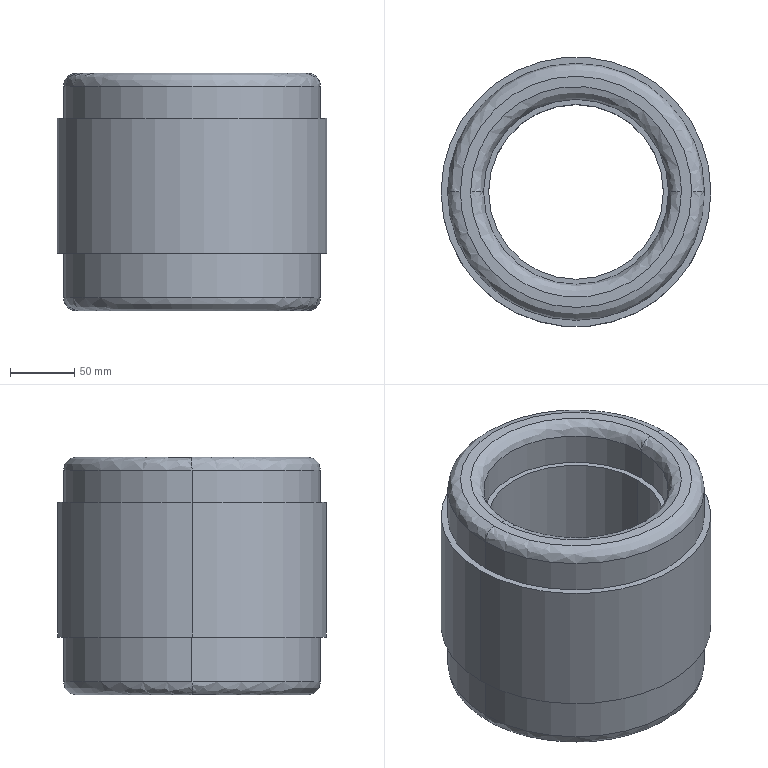Part | STEP file | 46 Coil | 1 solid | 26 faces | box 210 x 210 x 185 mm | volume 3277014 mm3 | cylinder 12 | spline 8 | plane 6 | commonest cylinder face diameters 144 x4 200 x4 136 x2 210 x2